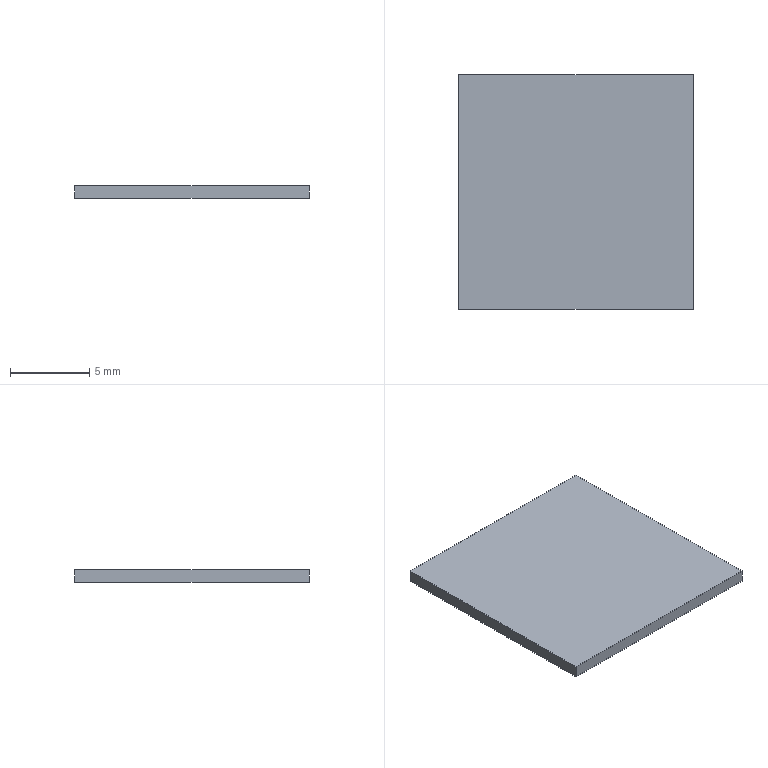Part | Creo | 1 solid | 6 faces | box 14.835 x 14.835 x 0.78 mm | volume 171.667 mm3 | plane 6
STEP:
#1=CARTESIAN_POINT('',(0.,0.,0.));
#2=DIRECTION('',(0.,0.,1.));
#3=DIRECTION('',(1.,0.,0.));
#4=AXIS2_PLACEMENT_3D('',#1,#2,#3);
#5=CARTESIAN_POINT('',(-7.418,-7.418,0.));
#6=VERTEX_POINT('',#5);
#7=CARTESIAN_POINT('',(7.418,-7.418,0.));
#8=VERTEX_POINT('',#7);
#9=CARTESIAN_POINT('',(-7.418,-7.418,0.));
#10=DIRECTION('',(1.,0.,0.));
#11=VECTOR('',#10,14.835);
#12=LINE('',#9,#11);
#13=EDGE_CURVE('',#6,#8,#12,.T.);
#14=ORIENTED_EDGE('',*,*,#13,.T.);
#15=CARTESIAN_POINT('',(7.418,7.418,0.));
#16=VERTEX_POINT('',#15);
#17=CARTESIAN_POINT('',(7.418,-7.418,0.));
#18=DIRECTION('',(0.,1.,0.));
#19=VECTOR('',#18,14.835);
#20=LINE('',#17,#19);
#21=EDGE_CURVE('',#8,#16,#20,.T.);
#22=ORIENTED_EDGE('',*,*,#21,.T.);
#23=CARTESIAN_POINT('',(-7.418,7.418,0.));
#24=VERTEX_POINT('',#23);
#25=CARTESIAN_POINT('',(7.418,7.418,0.));
#26=DIRECTION('',(-1.,0.,0.));
#27=VECTOR('',#26,14.835);
#28=LINE('',#25,#27);
#29=EDGE_CURVE('',#16,#24,#28,.T.);
#30=ORIENTED_EDGE('',*,*,#29,.T.);
#31=CARTESIAN_POINT('',(-7.418,7.418,0.));
#32=DIRECTION('',(0.,-1.,0.));
#33=VECTOR('',#32,14.835);
#34=LINE('',#31,#33);
#35=EDGE_CURVE('',#24,#6,#34,.T.);
#36=ORIENTED_EDGE('',*,*,#35,.T.);
#37=EDGE_LOOP('',(#14,#22,#30,#36));
#38=FACE_OUTER_BOUND('',#37,.F.);
#39=CARTESIAN_POINT('',(0.,0.,0.));
#40=DIRECTION('',(0.,0.,1.));
#41=DIRECTION('',(1.,0.,0.));
#42=AXIS2_PLACEMENT_3D('',#39,#40,#41);
#43=PLANE('',#42);
#44=ADVANCED_FACE('',(#38),#43,.F.);
#45=ORIENTED_EDGE('',*,*,#13,.F.);
#46=CARTESIAN_POINT('',(-7.418,-7.418,0.78));
#47=VERTEX_POINT('',#46);
#48=CARTESIAN_POINT('',(-7.418,-7.418,0.));
#49=DIRECTION('',(0.,0.,1.));
#50=VECTOR('',#49,0.78);
#51=LINE('',#48,#50);
#52=EDGE_CURVE('',#6,#47,#51,.T.);
#53=ORIENTED_EDGE('',*,*,#52,.T.);
#54=CARTESIAN_POINT('',(7.418,-7.418,0.78));
#55=VERTEX_POINT('',#54);
#56=CARTESIAN_POINT('',(-7.418,-7.418,0.78));
#57=DIRECTION('',(1.,0.,0.));
#58=VECTOR('',#57,14.835);
#59=LINE('',#56,#58);
#60=EDGE_CURVE('',#47,#55,#59,.T.);
#61=ORIENTED_EDGE('',*,*,#60,.T.);
#62=CARTESIAN_POINT('',(7.418,-7.418,0.));
#63=DIRECTION('',(0.,0.,1.));
#64=VECTOR('',#63,0.78);
#65=LINE('',#62,#64);
#66=EDGE_CURVE('',#8,#55,#65,.T.);
#67=ORIENTED_EDGE('',*,*,#66,.F.);
#68=EDGE_LOOP('',(#45,#53,#61,#67));
#69=FACE_OUTER_BOUND('',#68,.F.);
#70=CARTESIAN_POINT('',(-7.418,-7.418,0.));
#71=DIRECTION('',(0.,-1.,0.));
#72=DIRECTION('',(1.,0.,0.));
#73=AXIS2_PLACEMENT_3D('',#70,#71,#72);
#74=PLANE('',#73);
#75=ADVANCED_FACE('',(#69),#74,.T.);
#76=ORIENTED_EDGE('',*,*,#35,.F.);
#77=CARTESIAN_POINT('',(-7.418,7.418,0.78));
#78=VERTEX_POINT('',#77);
#79=CARTESIAN_POINT('',(-7.418,7.418,0.));
#80=DIRECTION('',(0.,0.,1.));
#81=VECTOR('',#80,0.78);
#82=LINE('',#79,#81);
#83=EDGE_CURVE('',#24,#78,#82,.T.);
#84=ORIENTED_EDGE('',*,*,#83,.T.);
#85=CARTESIAN_POINT('',(-7.418,7.418,0.78));
#86=DIRECTION('',(0.,-1.,0.));
#87=VECTOR('',#86,14.835);
#88=LINE('',#85,#87);
#89=EDGE_CURVE('',#78,#47,#88,.T.);
#90=ORIENTED_EDGE('',*,*,#89,.T.);
#91=ORIENTED_EDGE('',*,*,#52,.F.);
#92=EDGE_LOOP('',(#76,#84,#90,#91));
#93=FACE_OUTER_BOUND('',#92,.F.);
#94=CARTESIAN_POINT('',(-7.418,7.418,0.));
#95=DIRECTION('',(-1.,0.,0.));
#96=DIRECTION('',(0.,-1.,0.));
#97=AXIS2_PLACEMENT_3D('',#94,#95,#96);
#98=PLANE('',#97);
#99=ADVANCED_FACE('',(#93),#98,.T.);
#100=ORIENTED_EDGE('',*,*,#29,.F.);
#101=CARTESIAN_POINT('',(7.418,7.418,0.78));
#102=VERTEX_POINT('',#101);
#103=CARTESIAN_POINT('',(7.418,7.418,0.));
#104=DIRECTION('',(0.,0.,1.));
#105=VECTOR('',#104,0.78);
#106=LINE('',#103,#105);
#107=EDGE_CURVE('',#16,#102,#106,.T.);
#108=ORIENTED_EDGE('',*,*,#107,.T.);
#109=CARTESIAN_POINT('',(7.418,7.418,0.78));
#110=DIRECTION('',(-1.,0.,0.));
#111=VECTOR('',#110,14.835);
#112=LINE('',#109,#111);
#113=EDGE_CURVE('',#102,#78,#112,.T.);
#114=ORIENTED_EDGE('',*,*,#113,.T.);
#115=ORIENTED_EDGE('',*,*,#83,.F.);
#116=EDGE_LOOP('',(#100,#108,#114,#115));
#117=FACE_OUTER_BOUND('',#116,.F.);
#118=CARTESIAN_POINT('',(7.418,7.418,0.));
#119=DIRECTION('',(0.,1.,0.));
#120=DIRECTION('',(-1.,0.,0.));
#121=AXIS2_PLACEMENT_3D('',#118,#119,#120);
#122=PLANE('',#121);
#123=ADVANCED_FACE('',(#117),#122,.T.);
#124=ORIENTED_EDGE('',*,*,#21,.F.);
#125=ORIENTED_EDGE('',*,*,#66,.T.);
#126=CARTESIAN_POINT('',(7.418,-7.418,0.78));
#127=DIRECTION('',(0.,1.,0.));
#128=VECTOR('',#127,14.835);
#129=LINE('',#126,#128);
#130=EDGE_CURVE('',#55,#102,#129,.T.);
#131=ORIENTED_EDGE('',*,*,#130,.T.);
#132=ORIENTED_EDGE('',*,*,#107,.F.);
#133=EDGE_LOOP('',(#124,#125,#131,#132));
#134=FACE_OUTER_BOUND('',#133,.F.);
#135=CARTESIAN_POINT('',(7.418,-7.418,0.));
#136=DIRECTION('',(1.,0.,0.));
#137=DIRECTION('',(0.,1.,0.));
#138=AXIS2_PLACEMENT_3D('',#135,#136,#137);
#139=PLANE('',#138);
#140=ADVANCED_FACE('',(#134),#139,.T.);
#141=ORIENTED_EDGE('',*,*,#60,.F.);
#142=ORIENTED_EDGE('',*,*,#89,.F.);
#143=ORIENTED_EDGE('',*,*,#113,.F.);
#144=ORIENTED_EDGE('',*,*,#130,.F.);
#145=EDGE_LOOP('',(#141,#142,#143,#144));
#146=FACE_OUTER_BOUND('',#145,.F.);
#147=CARTESIAN_POINT('',(0.,0.,0.78));
#148=DIRECTION('',(0.,0.,1.));
#149=DIRECTION('',(1.,0.,0.));
#150=AXIS2_PLACEMENT_3D('',#147,#148,#149);
#151=PLANE('',#150);
#152=ADVANCED_FACE('',(#146),#151,.T.);
#153=CLOSED_SHELL('',(#44,#75,#99,#123,#140,#152));
#154=MANIFOLD_SOLID_BREP('',#153);
#155=(LENGTH_UNIT()NAMED_UNIT(*)SI_UNIT(.MILLI.,.METRE.));
#156=UNCERTAINTY_MEASURE_WITH_UNIT(LENGTH_MEASURE(0.002099),#155,'','');
#157=(NAMED_UNIT(*)PLANE_ANGLE_UNIT()SI_UNIT($,.RADIAN.));
#158=PLANE_ANGLE_MEASURE_WITH_UNIT(PLANE_ANGLE_MEASURE(0.01745),#157);
#159=(CONVERSION_BASED_UNIT('DEGREE',#158)NAMED_UNIT(*)PLANE_ANGLE_UNIT());
#160=(NAMED_UNIT(*)SI_UNIT($,.STERADIAN.)SOLID_ANGLE_UNIT());
#161=(GEOMETRIC_REPRESENTATION_CONTEXT(3)GLOBAL_UNCERTAINTY_ASSIGNED_CONTEXT((#156))GLOBAL_UNIT_ASSIGNED_CONTEXT((#155,#159,#160))REPRESENTATION_CONTEXT('',''));
#162=ADVANCED_BREP_SHAPE_REPRESENTATION('',(#4,#154),#161);